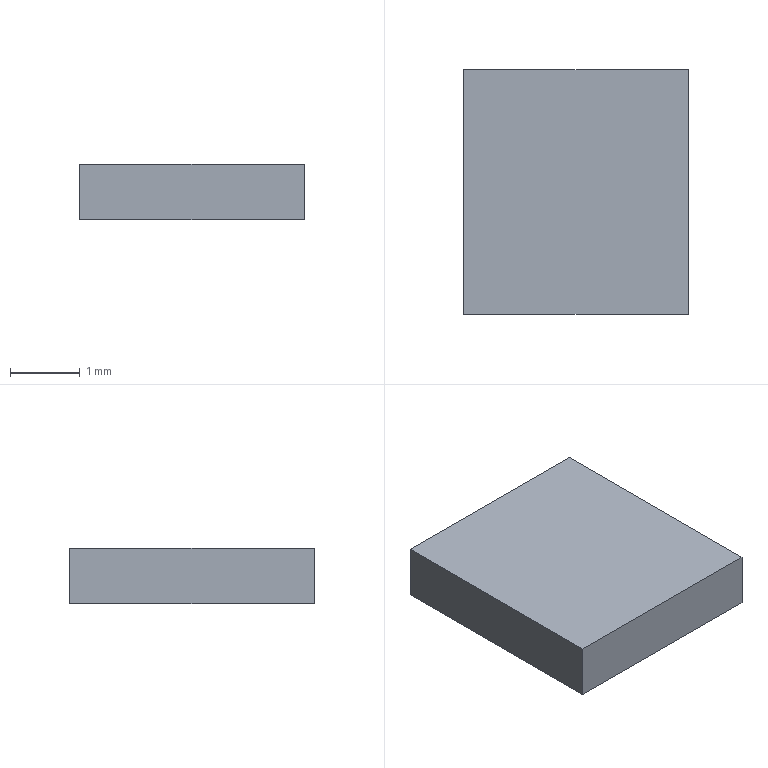Part | Creo | 1 solid | 6 faces | box 3.23 x 3.512 x 0.8 mm | volume 9.074 mm3 | plane 6
STEP:
#1=CARTESIAN_POINT('',(0.,0.,0.));
#2=DIRECTION('',(0.,0.,1.));
#3=DIRECTION('',(1.,0.,0.));
#4=AXIS2_PLACEMENT_3D('',#1,#2,#3);
#5=CARTESIAN_POINT('',(-1.655,-1.812,0.));
#6=VERTEX_POINT('',#5);
#7=CARTESIAN_POINT('',(1.575,-1.812,0.));
#8=VERTEX_POINT('',#7);
#9=CARTESIAN_POINT('',(-1.655,-1.812,0.));
#10=DIRECTION('',(1.,0.,0.));
#11=VECTOR('',#10,3.23);
#12=LINE('',#9,#11);
#13=EDGE_CURVE('',#6,#8,#12,.T.);
#14=ORIENTED_EDGE('',*,*,#13,.T.);
#15=CARTESIAN_POINT('',(1.575,1.7,0.));
#16=VERTEX_POINT('',#15);
#17=CARTESIAN_POINT('',(1.575,-1.812,0.));
#18=DIRECTION('',(0.,1.,0.));
#19=VECTOR('',#18,3.512);
#20=LINE('',#17,#19);
#21=EDGE_CURVE('',#8,#16,#20,.T.);
#22=ORIENTED_EDGE('',*,*,#21,.T.);
#23=CARTESIAN_POINT('',(-1.655,1.7,0.));
#24=VERTEX_POINT('',#23);
#25=CARTESIAN_POINT('',(1.575,1.7,0.));
#26=DIRECTION('',(-1.,0.,0.));
#27=VECTOR('',#26,3.23);
#28=LINE('',#25,#27);
#29=EDGE_CURVE('',#16,#24,#28,.T.);
#30=ORIENTED_EDGE('',*,*,#29,.T.);
#31=CARTESIAN_POINT('',(-1.655,1.7,0.));
#32=DIRECTION('',(0.,-1.,0.));
#33=VECTOR('',#32,3.512);
#34=LINE('',#31,#33);
#35=EDGE_CURVE('',#24,#6,#34,.T.);
#36=ORIENTED_EDGE('',*,*,#35,.T.);
#37=EDGE_LOOP('',(#14,#22,#30,#36));
#38=FACE_OUTER_BOUND('',#37,.F.);
#39=CARTESIAN_POINT('',(0.,0.,0.));
#40=DIRECTION('',(0.,0.,1.));
#41=DIRECTION('',(1.,0.,0.));
#42=AXIS2_PLACEMENT_3D('',#39,#40,#41);
#43=PLANE('',#42);
#44=ADVANCED_FACE('',(#38),#43,.F.);
#45=ORIENTED_EDGE('',*,*,#13,.F.);
#46=CARTESIAN_POINT('',(-1.655,-1.812,0.8));
#47=VERTEX_POINT('',#46);
#48=CARTESIAN_POINT('',(-1.655,-1.812,0.));
#49=DIRECTION('',(0.,0.,1.));
#50=VECTOR('',#49,0.8);
#51=LINE('',#48,#50);
#52=EDGE_CURVE('',#6,#47,#51,.T.);
#53=ORIENTED_EDGE('',*,*,#52,.T.);
#54=CARTESIAN_POINT('',(1.575,-1.812,0.8));
#55=VERTEX_POINT('',#54);
#56=CARTESIAN_POINT('',(-1.655,-1.812,0.8));
#57=DIRECTION('',(1.,0.,0.));
#58=VECTOR('',#57,3.23);
#59=LINE('',#56,#58);
#60=EDGE_CURVE('',#47,#55,#59,.T.);
#61=ORIENTED_EDGE('',*,*,#60,.T.);
#62=CARTESIAN_POINT('',(1.575,-1.812,0.));
#63=DIRECTION('',(0.,0.,1.));
#64=VECTOR('',#63,0.8);
#65=LINE('',#62,#64);
#66=EDGE_CURVE('',#8,#55,#65,.T.);
#67=ORIENTED_EDGE('',*,*,#66,.F.);
#68=EDGE_LOOP('',(#45,#53,#61,#67));
#69=FACE_OUTER_BOUND('',#68,.F.);
#70=CARTESIAN_POINT('',(-1.655,-1.812,0.));
#71=DIRECTION('',(0.,-1.,0.));
#72=DIRECTION('',(1.,0.,0.));
#73=AXIS2_PLACEMENT_3D('',#70,#71,#72);
#74=PLANE('',#73);
#75=ADVANCED_FACE('',(#69),#74,.T.);
#76=ORIENTED_EDGE('',*,*,#35,.F.);
#77=CARTESIAN_POINT('',(-1.655,1.7,0.8));
#78=VERTEX_POINT('',#77);
#79=CARTESIAN_POINT('',(-1.655,1.7,0.));
#80=DIRECTION('',(0.,0.,1.));
#81=VECTOR('',#80,0.8);
#82=LINE('',#79,#81);
#83=EDGE_CURVE('',#24,#78,#82,.T.);
#84=ORIENTED_EDGE('',*,*,#83,.T.);
#85=CARTESIAN_POINT('',(-1.655,1.7,0.8));
#86=DIRECTION('',(0.,-1.,0.));
#87=VECTOR('',#86,3.512);
#88=LINE('',#85,#87);
#89=EDGE_CURVE('',#78,#47,#88,.T.);
#90=ORIENTED_EDGE('',*,*,#89,.T.);
#91=ORIENTED_EDGE('',*,*,#52,.F.);
#92=EDGE_LOOP('',(#76,#84,#90,#91));
#93=FACE_OUTER_BOUND('',#92,.F.);
#94=CARTESIAN_POINT('',(-1.655,1.7,0.));
#95=DIRECTION('',(-1.,0.,0.));
#96=DIRECTION('',(0.,-1.,0.));
#97=AXIS2_PLACEMENT_3D('',#94,#95,#96);
#98=PLANE('',#97);
#99=ADVANCED_FACE('',(#93),#98,.T.);
#100=ORIENTED_EDGE('',*,*,#29,.F.);
#101=CARTESIAN_POINT('',(1.575,1.7,0.8));
#102=VERTEX_POINT('',#101);
#103=CARTESIAN_POINT('',(1.575,1.7,0.));
#104=DIRECTION('',(0.,0.,1.));
#105=VECTOR('',#104,0.8);
#106=LINE('',#103,#105);
#107=EDGE_CURVE('',#16,#102,#106,.T.);
#108=ORIENTED_EDGE('',*,*,#107,.T.);
#109=CARTESIAN_POINT('',(1.575,1.7,0.8));
#110=DIRECTION('',(-1.,0.,0.));
#111=VECTOR('',#110,3.23);
#112=LINE('',#109,#111);
#113=EDGE_CURVE('',#102,#78,#112,.T.);
#114=ORIENTED_EDGE('',*,*,#113,.T.);
#115=ORIENTED_EDGE('',*,*,#83,.F.);
#116=EDGE_LOOP('',(#100,#108,#114,#115));
#117=FACE_OUTER_BOUND('',#116,.F.);
#118=CARTESIAN_POINT('',(1.575,1.7,0.));
#119=DIRECTION('',(0.,1.,0.));
#120=DIRECTION('',(-1.,0.,0.));
#121=AXIS2_PLACEMENT_3D('',#118,#119,#120);
#122=PLANE('',#121);
#123=ADVANCED_FACE('',(#117),#122,.T.);
#124=ORIENTED_EDGE('',*,*,#21,.F.);
#125=ORIENTED_EDGE('',*,*,#66,.T.);
#126=CARTESIAN_POINT('',(1.575,-1.812,0.8));
#127=DIRECTION('',(0.,1.,0.));
#128=VECTOR('',#127,3.512);
#129=LINE('',#126,#128);
#130=EDGE_CURVE('',#55,#102,#129,.T.);
#131=ORIENTED_EDGE('',*,*,#130,.T.);
#132=ORIENTED_EDGE('',*,*,#107,.F.);
#133=EDGE_LOOP('',(#124,#125,#131,#132));
#134=FACE_OUTER_BOUND('',#133,.F.);
#135=CARTESIAN_POINT('',(1.575,-1.812,0.));
#136=DIRECTION('',(1.,0.,0.));
#137=DIRECTION('',(0.,1.,0.));
#138=AXIS2_PLACEMENT_3D('',#135,#136,#137);
#139=PLANE('',#138);
#140=ADVANCED_FACE('',(#134),#139,.T.);
#141=ORIENTED_EDGE('',*,*,#60,.F.);
#142=ORIENTED_EDGE('',*,*,#89,.F.);
#143=ORIENTED_EDGE('',*,*,#113,.F.);
#144=ORIENTED_EDGE('',*,*,#130,.F.);
#145=EDGE_LOOP('',(#141,#142,#143,#144));
#146=FACE_OUTER_BOUND('',#145,.F.);
#147=CARTESIAN_POINT('',(0.,0.,0.8));
#148=DIRECTION('',(0.,0.,1.));
#149=DIRECTION('',(1.,0.,0.));
#150=AXIS2_PLACEMENT_3D('',#147,#148,#149);
#151=PLANE('',#150);
#152=ADVANCED_FACE('',(#146),#151,.T.);
#153=CLOSED_SHELL('',(#44,#75,#99,#123,#140,#152));
#154=MANIFOLD_SOLID_BREP('',#153);
#155=(LENGTH_UNIT()NAMED_UNIT(*)SI_UNIT(.MILLI.,.METRE.));
#156=UNCERTAINTY_MEASURE_WITH_UNIT(LENGTH_MEASURE(0.0004838),#155,'','');
#157=(NAMED_UNIT(*)PLANE_ANGLE_UNIT()SI_UNIT($,.RADIAN.));
#158=PLANE_ANGLE_MEASURE_WITH_UNIT(PLANE_ANGLE_MEASURE(0.01745),#157);
#159=(CONVERSION_BASED_UNIT('DEGREE',#158)NAMED_UNIT(*)PLANE_ANGLE_UNIT());
#160=(NAMED_UNIT(*)SI_UNIT($,.STERADIAN.)SOLID_ANGLE_UNIT());
#161=(GEOMETRIC_REPRESENTATION_CONTEXT(3)GLOBAL_UNCERTAINTY_ASSIGNED_CONTEXT((#156))GLOBAL_UNIT_ASSIGNED_CONTEXT((#155,#159,#160))REPRESENTATION_CONTEXT('',''));
#162=ADVANCED_BREP_SHAPE_REPRESENTATION('',(#4,#154),#161);